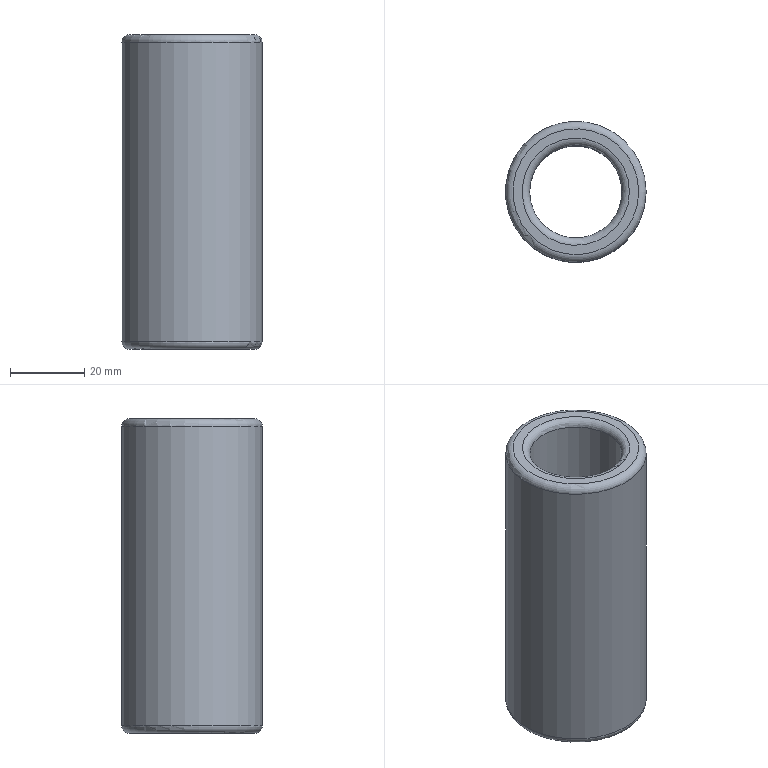Part | NX | features DATUM_CSYS 2, BLEND 1, EXTRUDE 1, SKETCH 1 | 1 solid | 8 faces | box 38 x 38 x 85 mm | volume 54336 mm3 | torus 4 | cylinder 2 | plane 2 | commonest cylinder face diameters 25 x1 38 x1
STEP:
#1=CARTESIAN_POINT('',(19.,0.,2.));
#2=VERTEX_POINT('',#1);
#3=CARTESIAN_POINT('',(0.,0.,2.));
#4=DIRECTION('',(0.,0.,1.));
#5=DIRECTION('',(1.,0.,0.));
#6=AXIS2_PLACEMENT_3D('',#3,#4,#5);
#7=CIRCLE('',#6,19.);
#8=EDGE_CURVE('',#2,#2,#7,.T.);
#9=ORIENTED_EDGE('',*,*,#8,.T.);
#10=EDGE_LOOP('',(#9));
#11=FACE_BOUND('',#10,.T.);
#12=CARTESIAN_POINT('',(19.,0.,83.));
#13=VERTEX_POINT('',#12);
#14=CARTESIAN_POINT('',(0.,0.,83.));
#15=DIRECTION('',(0.,0.,1.));
#16=DIRECTION('',(1.,0.,0.));
#17=AXIS2_PLACEMENT_3D('',#14,#15,#16);
#18=CIRCLE('',#17,19.);
#19=EDGE_CURVE('',#13,#13,#18,.F.);
#20=ORIENTED_EDGE('',*,*,#19,.T.);
#21=EDGE_LOOP('',(#20));
#22=FACE_BOUND('',#21,.T.);
#23=CARTESIAN_POINT('',(0.,0.,85.));
#24=DIRECTION('',(0.,0.,-1.));
#25=DIRECTION('',(-1.,0.,0.));
#26=AXIS2_PLACEMENT_3D('',#23,#24,#25);
#27=CYLINDRICAL_SURFACE('',#26,19.);
#28=ADVANCED_FACE('',(#11,#22),#27,.T.);
#29=CARTESIAN_POINT('',(12.5,0.,2.));
#30=VERTEX_POINT('',#29);
#31=CARTESIAN_POINT('',(0.,0.,2.));
#32=DIRECTION('',(0.,0.,1.));
#33=DIRECTION('',(1.,0.,0.));
#34=AXIS2_PLACEMENT_3D('',#31,#32,#33);
#35=CIRCLE('',#34,12.5);
#36=EDGE_CURVE('',#30,#30,#35,.F.);
#37=ORIENTED_EDGE('',*,*,#36,.T.);
#38=EDGE_LOOP('',(#37));
#39=FACE_BOUND('',#38,.T.);
#40=CARTESIAN_POINT('',(12.5,0.,83.));
#41=VERTEX_POINT('',#40);
#42=CARTESIAN_POINT('',(0.,0.,83.));
#43=DIRECTION('',(0.,0.,1.));
#44=DIRECTION('',(1.,0.,0.));
#45=AXIS2_PLACEMENT_3D('',#42,#43,#44);
#46=CIRCLE('',#45,12.5);
#47=EDGE_CURVE('',#41,#41,#46,.T.);
#48=ORIENTED_EDGE('',*,*,#47,.T.);
#49=EDGE_LOOP('',(#48));
#50=FACE_BOUND('',#49,.T.);
#51=CARTESIAN_POINT('',(0.,0.,85.));
#52=DIRECTION('',(0.,0.,-1.));
#53=DIRECTION('',(-1.,0.,0.));
#54=AXIS2_PLACEMENT_3D('',#51,#52,#53);
#55=CYLINDRICAL_SURFACE('',#54,12.5);
#56=ADVANCED_FACE('',(#39,#50),#55,.F.);
#57=CARTESIAN_POINT('',(17.,0.,85.));
#58=VERTEX_POINT('',#57);
#59=CARTESIAN_POINT('',(0.,0.,85.));
#60=DIRECTION('',(0.,0.,1.));
#61=DIRECTION('',(1.,0.,0.));
#62=AXIS2_PLACEMENT_3D('',#59,#60,#61);
#63=CIRCLE('',#62,17.);
#64=EDGE_CURVE('',#58,#58,#63,.T.);
#65=ORIENTED_EDGE('',*,*,#64,.T.);
#66=EDGE_LOOP('',(#65));
#67=FACE_BOUND('',#66,.T.);
#68=CARTESIAN_POINT('',(14.5,0.,85.));
#69=VERTEX_POINT('',#68);
#70=CARTESIAN_POINT('',(0.,0.,85.));
#71=DIRECTION('',(0.,0.,1.));
#72=DIRECTION('',(1.,0.,0.));
#73=AXIS2_PLACEMENT_3D('',#70,#71,#72);
#74=CIRCLE('',#73,14.5);
#75=EDGE_CURVE('',#69,#69,#74,.F.);
#76=ORIENTED_EDGE('',*,*,#75,.T.);
#77=EDGE_LOOP('',(#76));
#78=FACE_BOUND('',#77,.T.);
#79=CARTESIAN_POINT('',(0.,0.,85.));
#80=DIRECTION('',(0.,0.,1.));
#81=DIRECTION('',(1.,0.,0.));
#82=AXIS2_PLACEMENT_3D('',#79,#80,#81);
#83=PLANE('',#82);
#84=ADVANCED_FACE('',(#67,#78),#83,.T.);
#85=CARTESIAN_POINT('',(14.5,0.,0.));
#86=VERTEX_POINT('',#85);
#87=CARTESIAN_POINT('',(0.,0.,0.));
#88=DIRECTION('',(0.,0.,1.));
#89=DIRECTION('',(1.,0.,0.));
#90=AXIS2_PLACEMENT_3D('',#87,#88,#89);
#91=CIRCLE('',#90,14.5);
#92=EDGE_CURVE('',#86,#86,#91,.T.);
#93=ORIENTED_EDGE('',*,*,#92,.T.);
#94=EDGE_LOOP('',(#93));
#95=FACE_BOUND('',#94,.T.);
#96=CARTESIAN_POINT('',(17.,0.,0.));
#97=VERTEX_POINT('',#96);
#98=CARTESIAN_POINT('',(0.,0.,0.));
#99=DIRECTION('',(0.,0.,1.));
#100=DIRECTION('',(1.,0.,0.));
#101=AXIS2_PLACEMENT_3D('',#98,#99,#100);
#102=CIRCLE('',#101,17.);
#103=EDGE_CURVE('',#97,#97,#102,.F.);
#104=ORIENTED_EDGE('',*,*,#103,.T.);
#105=EDGE_LOOP('',(#104));
#106=FACE_BOUND('',#105,.T.);
#107=CARTESIAN_POINT('',(0.,0.,0.));
#108=DIRECTION('',(0.,0.,1.));
#109=DIRECTION('',(1.,0.,0.));
#110=AXIS2_PLACEMENT_3D('',#107,#108,#109);
#111=PLANE('',#110);
#112=ADVANCED_FACE('',(#95,#106),#111,.F.);
#113=ORIENTED_EDGE('',*,*,#36,.F.);
#114=EDGE_LOOP('',(#113));
#115=FACE_BOUND('',#114,.T.);
#116=ORIENTED_EDGE('',*,*,#92,.F.);
#117=EDGE_LOOP('',(#116));
#118=FACE_BOUND('',#117,.T.);
#119=CARTESIAN_POINT('',(0.,0.,2.));
#120=DIRECTION('',(0.,0.,1.));
#121=DIRECTION('',(1.,0.,0.));
#122=AXIS2_PLACEMENT_3D('',#119,#120,#121);
#123=TOROIDAL_SURFACE('',#122,14.5,2.);
#124=ADVANCED_FACE('',(#115,#118),#123,.T.);
#125=ORIENTED_EDGE('',*,*,#103,.F.);
#126=EDGE_LOOP('',(#125));
#127=FACE_BOUND('',#126,.T.);
#128=ORIENTED_EDGE('',*,*,#8,.F.);
#129=EDGE_LOOP('',(#128));
#130=FACE_BOUND('',#129,.T.);
#131=CARTESIAN_POINT('',(0.,0.,2.));
#132=DIRECTION('',(0.,0.,1.));
#133=DIRECTION('',(1.,0.,0.));
#134=AXIS2_PLACEMENT_3D('',#131,#132,#133);
#135=TOROIDAL_SURFACE('',#134,17.,2.);
#136=ADVANCED_FACE('',(#127,#130),#135,.T.);
#137=ORIENTED_EDGE('',*,*,#19,.F.);
#138=EDGE_LOOP('',(#137));
#139=FACE_BOUND('',#138,.T.);
#140=ORIENTED_EDGE('',*,*,#64,.F.);
#141=EDGE_LOOP('',(#140));
#142=FACE_BOUND('',#141,.T.);
#143=CARTESIAN_POINT('',(0.,0.,83.));
#144=DIRECTION('',(0.,0.,1.));
#145=DIRECTION('',(1.,0.,0.));
#146=AXIS2_PLACEMENT_3D('',#143,#144,#145);
#147=TOROIDAL_SURFACE('',#146,17.,2.);
#148=ADVANCED_FACE('',(#139,#142),#147,.T.);
#149=ORIENTED_EDGE('',*,*,#75,.F.);
#150=EDGE_LOOP('',(#149));
#151=FACE_BOUND('',#150,.T.);
#152=ORIENTED_EDGE('',*,*,#47,.F.);
#153=EDGE_LOOP('',(#152));
#154=FACE_BOUND('',#153,.T.);
#155=CARTESIAN_POINT('',(0.,0.,83.));
#156=DIRECTION('',(0.,0.,1.));
#157=DIRECTION('',(1.,0.,0.));
#158=AXIS2_PLACEMENT_3D('',#155,#156,#157);
#159=TOROIDAL_SURFACE('',#158,14.5,2.);
#160=ADVANCED_FACE('',(#151,#154),#159,.T.);
#161=CLOSED_SHELL('',(#28,#56,#84,#112,#124,#136,#148,#160));
#162=MANIFOLD_SOLID_BREP('',#161);
#163=(LENGTH_UNIT()NAMED_UNIT(*)SI_UNIT(.MILLI.,.METRE.));
#164=UNCERTAINTY_MEASURE_WITH_UNIT(LENGTH_MEASURE(0.00001),#163,'','');
#165=(NAMED_UNIT(*)PLANE_ANGLE_UNIT()SI_UNIT($,.RADIAN.));
#166=(NAMED_UNIT(*)SI_UNIT($,.STERADIAN.)SOLID_ANGLE_UNIT());
#167=(GEOMETRIC_REPRESENTATION_CONTEXT(3)GLOBAL_UNCERTAINTY_ASSIGNED_CONTEXT((#164))GLOBAL_UNIT_ASSIGNED_CONTEXT((#163,#165,#166))REPRESENTATION_CONTEXT('',''));
#168=ADVANCED_BREP_SHAPE_REPRESENTATION('',(#162),#167);